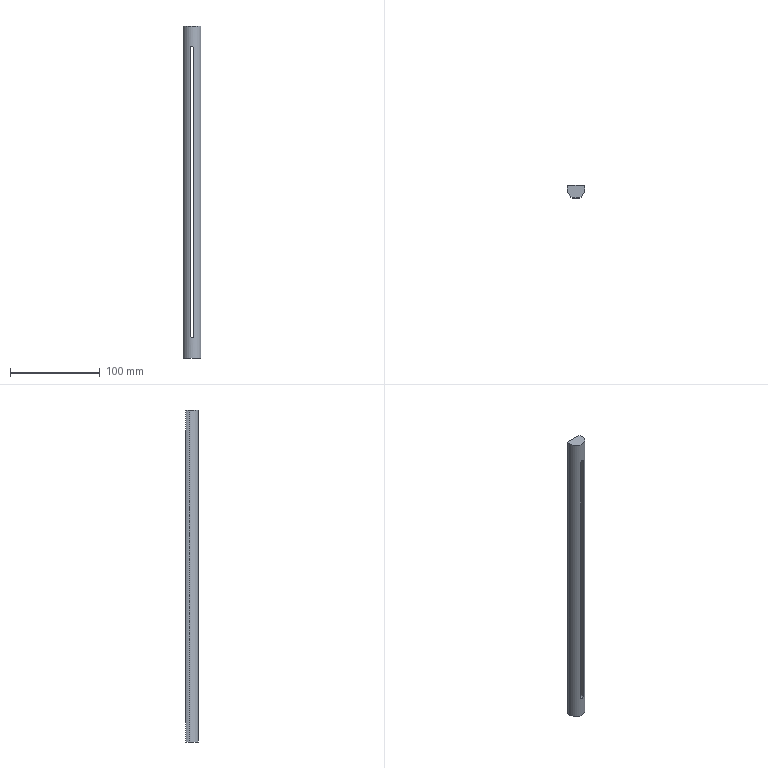Part | SolidWorks | features ICE 2, Extrusion 1 | 1 solid | 11 faces | box 20 x 14 x 370 mm | volume 68901 mm3 | cylinder 6 | plane 5 | commonest cylinder face diameters 4 x3 20 x3
STEP:
#1=CARTESIAN_POINT('',(0.,-10.,162.));
#2=VERTEX_POINT('',#1);
#3=CARTESIAN_POINT('',(2.,-9.798,160.));
#4=VERTEX_POINT('',#3);
#5=CARTESIAN_POINT('',(0.,-10.,162.));
#6=CARTESIAN_POINT('',(0.1307,-10.,162.));
#7=CARTESIAN_POINT('',(0.2635,-9.997,161.987));
#8=CARTESIAN_POINT('',(0.5201,-9.987,161.936));
#9=CARTESIAN_POINT('',(0.6448,-9.98,161.898));
#10=CARTESIAN_POINT('',(1.008,-9.952,161.747));
#11=CARTESIAN_POINT('',(1.228,-9.926,161.6));
#12=CARTESIAN_POINT('',(1.507,-9.886,161.322));
#13=CARTESIAN_POINT('',(1.589,-9.873,161.221));
#14=CARTESIAN_POINT('',(1.734,-9.849,161.005));
#15=CARTESIAN_POINT('',(1.797,-9.837,160.888));
#16=CARTESIAN_POINT('',(1.897,-9.819,160.646));
#17=CARTESIAN_POINT('',(1.935,-9.811,160.522));
#18=CARTESIAN_POINT('',(1.987,-9.801,160.265));
#19=CARTESIAN_POINT('',(2.,-9.798,160.132));
#20=CARTESIAN_POINT('',(2.,-9.798,160.));
#21=B_SPLINE_CURVE_WITH_KNOTS('',3,(#5,#6,#7,#8,#9,#10,#11,#12,#13,#14,#15,#16,#17,#18,#19,#20),.UNSPECIFIED.,.F.,.F.,(4,2,2,2,2,2,2,4),(0.003135,0.003527,0.003918,0.004701,0.005093,0.005484,0.005876,0.006267),.UNSPECIFIED.);
#22=EDGE_CURVE('',#2,#4,#21,.T.);
#23=ORIENTED_EDGE('',*,*,#22,.F.);
#24=CARTESIAN_POINT('',(0.,4.,162.));
#25=VERTEX_POINT('',#24);
#26=CARTESIAN_POINT('',(0.,-12.5,162.));
#27=DIRECTION('',(0.,1.,0.));
#28=VECTOR('',#27,1000.);
#29=LINE('',#26,#28);
#30=EDGE_CURVE('',#2,#25,#29,.T.);
#31=ORIENTED_EDGE('',*,*,#30,.T.);
#32=CARTESIAN_POINT('',(2.,4.,160.));
#33=VERTEX_POINT('',#32);
#34=CARTESIAN_POINT('',(0.,4.,160.));
#35=DIRECTION('',(0.,1.,0.));
#36=DIRECTION('',(0.,0.,-1.));
#37=AXIS2_PLACEMENT_3D('',#34,#35,#36);
#38=CIRCLE('',#37,2.);
#39=EDGE_CURVE('',#25,#33,#38,.T.);
#40=ORIENTED_EDGE('',*,*,#39,.T.);
#41=CARTESIAN_POINT('',(2.,-12.5,160.));
#42=DIRECTION('',(0.,1.,0.));
#43=VECTOR('',#42,1000.);
#44=LINE('',#41,#43);
#45=EDGE_CURVE('',#4,#33,#44,.T.);
#46=ORIENTED_EDGE('',*,*,#45,.F.);
#47=EDGE_LOOP('',(#23,#31,#40,#46));
#48=FACE_OUTER_BOUND('',#47,.T.);
#49=CARTESIAN_POINT('',(0.,-12.5,160.));
#50=DIRECTION('',(0.,1.,0.));
#51=DIRECTION('',(0.,0.,1.));
#52=AXIS2_PLACEMENT_3D('',#49,#50,#51);
#53=CYLINDRICAL_SURFACE('',#52,2.);
#54=ADVANCED_FACE('',(#48),#53,.F.);
#55=CARTESIAN_POINT('',(10.,0.,185.));
#56=VERTEX_POINT('',#55);
#57=CARTESIAN_POINT('',(9.165,4.,185.));
#58=VERTEX_POINT('',#57);
#59=CARTESIAN_POINT('',(0.,0.,185.));
#60=DIRECTION('',(0.,0.,1.));
#61=DIRECTION('',(1.,0.,0.));
#62=AXIS2_PLACEMENT_3D('',#59,#60,#61);
#63=CIRCLE('',#62,10.);
#64=EDGE_CURVE('',#56,#58,#63,.T.);
#65=ORIENTED_EDGE('',*,*,#64,.F.);
#66=CARTESIAN_POINT('',(10.,0.,-185.));
#67=VERTEX_POINT('',#66);
#68=CARTESIAN_POINT('',(10.,0.,185.));
#69=DIRECTION('',(0.,0.,-1.));
#70=VECTOR('',#69,1000.);
#71=LINE('',#68,#70);
#72=EDGE_CURVE('',#56,#67,#71,.T.);
#73=ORIENTED_EDGE('',*,*,#72,.T.);
#74=CARTESIAN_POINT('',(9.165,4.,-185.));
#75=VERTEX_POINT('',#74);
#76=CARTESIAN_POINT('',(0.,0.,-185.));
#77=DIRECTION('',(0.,0.,1.));
#78=DIRECTION('',(1.,0.,0.));
#79=AXIS2_PLACEMENT_3D('',#76,#77,#78);
#80=CIRCLE('',#79,10.);
#81=EDGE_CURVE('',#67,#75,#80,.T.);
#82=ORIENTED_EDGE('',*,*,#81,.T.);
#83=CARTESIAN_POINT('',(9.165,4.,185.));
#84=DIRECTION('',(0.,0.,1.));
#85=VECTOR('',#84,1000.);
#86=LINE('',#83,#85);
#87=EDGE_CURVE('',#75,#58,#86,.T.);
#88=ORIENTED_EDGE('',*,*,#87,.T.);
#89=EDGE_LOOP('',(#65,#73,#82,#88));
#90=FACE_OUTER_BOUND('',#89,.T.);
#91=CARTESIAN_POINT('',(0.,0.,185.));
#92=DIRECTION('',(0.,0.,-1.));
#93=DIRECTION('',(-1.,0.,0.));
#94=AXIS2_PLACEMENT_3D('',#91,#92,#93);
#95=CYLINDRICAL_SURFACE('',#94,10.);
#96=ADVANCED_FACE('',(#90),#95,.T.);
#97=ORIENTED_EDGE('',*,*,#72,.F.);
#98=CARTESIAN_POINT('',(-10.,0.,185.));
#99=VERTEX_POINT('',#98);
#100=CARTESIAN_POINT('',(0.,0.,185.));
#101=DIRECTION('',(0.,0.,1.));
#102=DIRECTION('',(1.,0.,0.));
#103=AXIS2_PLACEMENT_3D('',#100,#101,#102);
#104=CIRCLE('',#103,10.);
#105=EDGE_CURVE('',#99,#56,#104,.T.);
#106=ORIENTED_EDGE('',*,*,#105,.F.);
#107=CARTESIAN_POINT('',(-10.,0.,-185.));
#108=VERTEX_POINT('',#107);
#109=CARTESIAN_POINT('',(-10.,0.,185.));
#110=DIRECTION('',(0.,0.,-1.));
#111=VECTOR('',#110,1000.);
#112=LINE('',#109,#111);
#113=EDGE_CURVE('',#99,#108,#112,.T.);
#114=ORIENTED_EDGE('',*,*,#113,.T.);
#115=CARTESIAN_POINT('',(0.,0.,-185.));
#116=DIRECTION('',(0.,0.,1.));
#117=DIRECTION('',(1.,0.,0.));
#118=AXIS2_PLACEMENT_3D('',#115,#116,#117);
#119=CIRCLE('',#118,10.);
#120=EDGE_CURVE('',#108,#67,#119,.T.);
#121=ORIENTED_EDGE('',*,*,#120,.T.);
#122=EDGE_LOOP('',(#97,#106,#114,#121));
#123=FACE_OUTER_BOUND('',#122,.T.);
#124=CARTESIAN_POINT('',(-2.,-9.798,-160.));
#125=VERTEX_POINT('',#124);
#126=CARTESIAN_POINT('',(-2.,-9.798,160.));
#127=VERTEX_POINT('',#126);
#128=CARTESIAN_POINT('',(-2.,-9.798,185.));
#129=DIRECTION('',(0.,0.,1.));
#130=VECTOR('',#129,1000.);
#131=LINE('',#128,#130);
#132=EDGE_CURVE('',#125,#127,#131,.T.);
#133=ORIENTED_EDGE('',*,*,#132,.T.);
#134=CARTESIAN_POINT('',(-2.,-9.798,160.));
#135=CARTESIAN_POINT('',(-2.,-9.798,160.133));
#136=CARTESIAN_POINT('',(-1.987,-9.801,160.263));
#137=CARTESIAN_POINT('',(-1.936,-9.811,160.519));
#138=CARTESIAN_POINT('',(-1.897,-9.819,160.646));
#139=CARTESIAN_POINT('',(-1.797,-9.837,160.888));
#140=CARTESIAN_POINT('',(-1.735,-9.849,161.003));
#141=CARTESIAN_POINT('',(-1.59,-9.873,161.22));
#142=CARTESIAN_POINT('',(-1.506,-9.886,161.323));
#143=CARTESIAN_POINT('',(-1.23,-9.926,161.599));
#144=CARTESIAN_POINT('',(-1.007,-9.952,161.748));
#145=CARTESIAN_POINT('',(-0.5255,-9.989,161.947));
#146=CARTESIAN_POINT('',(-0.2617,-10.,162.));
#147=CARTESIAN_POINT('',(0.,-10.,162.));
#148=B_SPLINE_CURVE_WITH_KNOTS('',3,(#134,#135,#136,#137,#138,#139,#140,#141,#142,#143,#144,#145,#146,#147),.UNSPECIFIED.,.F.,.F.,(4,2,2,2,2,2,4),(0.,0.0003919,0.0007838,0.001176,0.001568,0.002351,0.003135),.UNSPECIFIED.);
#149=EDGE_CURVE('',#127,#2,#148,.T.);
#150=ORIENTED_EDGE('',*,*,#149,.T.);
#151=ORIENTED_EDGE('',*,*,#22,.T.);
#152=CARTESIAN_POINT('',(2.,-9.798,-160.));
#153=VERTEX_POINT('',#152);
#154=CARTESIAN_POINT('',(2.,-9.798,185.));
#155=DIRECTION('',(0.,0.,-1.));
#156=VECTOR('',#155,1000.);
#157=LINE('',#154,#156);
#158=EDGE_CURVE('',#4,#153,#157,.T.);
#159=ORIENTED_EDGE('',*,*,#158,.T.);
#160=CARTESIAN_POINT('',(2.,-9.798,-160.));
#161=CARTESIAN_POINT('',(2.,-9.798,-160.132));
#162=CARTESIAN_POINT('',(1.987,-9.801,-160.263));
#163=CARTESIAN_POINT('',(1.936,-9.811,-160.519));
#164=CARTESIAN_POINT('',(1.897,-9.818,-160.646));
#165=CARTESIAN_POINT('',(1.797,-9.837,-160.888));
#166=CARTESIAN_POINT('',(1.735,-9.849,-161.003));
#167=CARTESIAN_POINT('',(1.59,-9.873,-161.22));
#168=CARTESIAN_POINT('',(1.506,-9.886,-161.322));
#169=CARTESIAN_POINT('',(1.23,-9.926,-161.598));
#170=CARTESIAN_POINT('',(1.008,-9.952,-161.747));
#171=CARTESIAN_POINT('',(0.5268,-9.989,-161.947));
#172=CARTESIAN_POINT('',(0.2632,-10.,-162.));
#173=CARTESIAN_POINT('',(-0.1292,-10.,-162.));
#174=CARTESIAN_POINT('',(-0.262,-9.997,-161.987));
#175=CARTESIAN_POINT('',(-0.5188,-9.987,-161.936));
#176=CARTESIAN_POINT('',(-0.6436,-9.98,-161.898));
#177=CARTESIAN_POINT('',(-1.007,-9.952,-161.748));
#178=CARTESIAN_POINT('',(-1.228,-9.926,-161.601));
#179=CARTESIAN_POINT('',(-1.506,-9.886,-161.322));
#180=CARTESIAN_POINT('',(-1.589,-9.873,-161.221));
#181=CARTESIAN_POINT('',(-1.734,-9.849,-161.005));
#182=CARTESIAN_POINT('',(-1.797,-9.837,-160.888));
#183=CARTESIAN_POINT('',(-1.897,-9.819,-160.647));
#184=CARTESIAN_POINT('',(-1.935,-9.811,-160.522));
#185=CARTESIAN_POINT('',(-1.987,-9.801,-160.265));
#186=CARTESIAN_POINT('',(-2.,-9.798,-160.132));
#187=CARTESIAN_POINT('',(-2.,-9.798,-160.));
#188=B_SPLINE_CURVE_WITH_KNOTS('',3,(#160,#161,#162,#163,#164,#165,#166,#167,#168,#169,#170,#171,#172,#173,#174,#175,#176,#177,#178,#179,#180,#181,#182,#183,#184,#185,#186,#187),.UNSPECIFIED.,.F.,.F.,(4,2,2,2,2,2,2,2,2,2,2,2,2,4),(0.,0.0003917,0.0007834,0.001175,0.001567,0.00235,0.003134,0.003525,0.003917,0.0047,0.005092,0.005484,0.005875,0.006267),.UNSPECIFIED.);
#189=EDGE_CURVE('',#153,#125,#188,.T.);
#190=ORIENTED_EDGE('',*,*,#189,.T.);
#191=EDGE_LOOP('',(#133,#150,#151,#159,#190));
#192=FACE_BOUND('',#191,.T.);
#193=CARTESIAN_POINT('',(0.,0.,185.));
#194=DIRECTION('',(0.,0.,-1.));
#195=DIRECTION('',(-1.,0.,0.));
#196=AXIS2_PLACEMENT_3D('',#193,#194,#195);
#197=CYLINDRICAL_SURFACE('',#196,10.);
#198=ADVANCED_FACE('',(#123,#192),#197,.T.);
#199=ORIENTED_EDGE('',*,*,#113,.F.);
#200=CARTESIAN_POINT('',(-9.165,4.,185.));
#201=VERTEX_POINT('',#200);
#202=CARTESIAN_POINT('',(0.,0.,185.));
#203=DIRECTION('',(0.,0.,1.));
#204=DIRECTION('',(1.,0.,0.));
#205=AXIS2_PLACEMENT_3D('',#202,#203,#204);
#206=CIRCLE('',#205,10.);
#207=EDGE_CURVE('',#201,#99,#206,.T.);
#208=ORIENTED_EDGE('',*,*,#207,.F.);
#209=CARTESIAN_POINT('',(-9.165,4.,-185.));
#210=VERTEX_POINT('',#209);
#211=CARTESIAN_POINT('',(-9.165,4.,185.));
#212=DIRECTION('',(0.,0.,-1.));
#213=VECTOR('',#212,1000.);
#214=LINE('',#211,#213);
#215=EDGE_CURVE('',#201,#210,#214,.T.);
#216=ORIENTED_EDGE('',*,*,#215,.T.);
#217=CARTESIAN_POINT('',(0.,0.,-185.));
#218=DIRECTION('',(0.,0.,1.));
#219=DIRECTION('',(1.,0.,0.));
#220=AXIS2_PLACEMENT_3D('',#217,#218,#219);
#221=CIRCLE('',#220,10.);
#222=EDGE_CURVE('',#210,#108,#221,.T.);
#223=ORIENTED_EDGE('',*,*,#222,.T.);
#224=EDGE_LOOP('',(#199,#208,#216,#223));
#225=FACE_OUTER_BOUND('',#224,.T.);
#226=CARTESIAN_POINT('',(0.,0.,185.));
#227=DIRECTION('',(0.,0.,-1.));
#228=DIRECTION('',(-1.,0.,0.));
#229=AXIS2_PLACEMENT_3D('',#226,#227,#228);
#230=CYLINDRICAL_SURFACE('',#229,10.);
#231=ADVANCED_FACE('',(#225),#230,.T.);
#232=CARTESIAN_POINT('',(-10.,4.,185.));
#233=DIRECTION('',(1.,0.,0.));
#234=VECTOR('',#233,1000.);
#235=LINE('',#232,#234);
#236=EDGE_CURVE('',#201,#58,#235,.T.);
#237=ORIENTED_EDGE('',*,*,#236,.F.);
#238=ORIENTED_EDGE('',*,*,#207,.T.);
#239=ORIENTED_EDGE('',*,*,#105,.T.);
#240=ORIENTED_EDGE('',*,*,#64,.T.);
#241=EDGE_LOOP('',(#237,#238,#239,#240));
#242=FACE_OUTER_BOUND('',#241,.T.);
#243=CARTESIAN_POINT('',(0.,0.,185.));
#244=DIRECTION('',(0.,0.,1.));
#245=DIRECTION('',(1.,0.,0.));
#246=AXIS2_PLACEMENT_3D('',#243,#244,#245);
#247=PLANE('',#246);
#248=ADVANCED_FACE('',(#242),#247,.T.);
#249=ORIENTED_EDGE('',*,*,#222,.F.);
#250=CARTESIAN_POINT('',(-10.,4.,-185.));
#251=DIRECTION('',(1.,0.,0.));
#252=VECTOR('',#251,1000.);
#253=LINE('',#250,#252);
#254=EDGE_CURVE('',#210,#75,#253,.T.);
#255=ORIENTED_EDGE('',*,*,#254,.T.);
#256=ORIENTED_EDGE('',*,*,#81,.F.);
#257=ORIENTED_EDGE('',*,*,#120,.F.);
#258=EDGE_LOOP('',(#249,#255,#256,#257));
#259=FACE_OUTER_BOUND('',#258,.T.);
#260=CARTESIAN_POINT('',(0.,0.,-185.));
#261=DIRECTION('',(0.,0.,1.));
#262=DIRECTION('',(1.,0.,0.));
#263=AXIS2_PLACEMENT_3D('',#260,#261,#262);
#264=PLANE('',#263);
#265=ADVANCED_FACE('',(#259),#264,.F.);
#266=ORIENTED_EDGE('',*,*,#30,.F.);
#267=ORIENTED_EDGE('',*,*,#149,.F.);
#268=CARTESIAN_POINT('',(-2.,4.,160.));
#269=VERTEX_POINT('',#268);
#270=CARTESIAN_POINT('',(-2.,-12.5,160.));
#271=DIRECTION('',(0.,1.,0.));
#272=VECTOR('',#271,1000.);
#273=LINE('',#270,#272);
#274=EDGE_CURVE('',#127,#269,#273,.T.);
#275=ORIENTED_EDGE('',*,*,#274,.T.);
#276=CARTESIAN_POINT('',(0.,4.,160.));
#277=DIRECTION('',(0.,1.,0.));
#278=DIRECTION('',(0.,0.,-1.));
#279=AXIS2_PLACEMENT_3D('',#276,#277,#278);
#280=CIRCLE('',#279,2.);
#281=EDGE_CURVE('',#269,#25,#280,.T.);
#282=ORIENTED_EDGE('',*,*,#281,.T.);
#283=EDGE_LOOP('',(#266,#267,#275,#282));
#284=FACE_OUTER_BOUND('',#283,.T.);
#285=CARTESIAN_POINT('',(0.,-12.5,160.));
#286=DIRECTION('',(0.,1.,0.));
#287=DIRECTION('',(0.,0.,1.));
#288=AXIS2_PLACEMENT_3D('',#285,#286,#287);
#289=CYLINDRICAL_SURFACE('',#288,2.);
#290=ADVANCED_FACE('',(#284),#289,.F.);
#291=CARTESIAN_POINT('',(-2.,4.,-160.));
#292=VERTEX_POINT('',#291);
#293=CARTESIAN_POINT('',(-2.,-12.5,-160.));
#294=DIRECTION('',(0.,1.,0.));
#295=VECTOR('',#294,1000.);
#296=LINE('',#293,#295);
#297=EDGE_CURVE('',#125,#292,#296,.T.);
#298=ORIENTED_EDGE('',*,*,#297,.T.);
#299=CARTESIAN_POINT('',(-2.,4.,160.));
#300=DIRECTION('',(0.,0.,1.));
#301=VECTOR('',#300,1000.);
#302=LINE('',#299,#301);
#303=EDGE_CURVE('',#292,#269,#302,.T.);
#304=ORIENTED_EDGE('',*,*,#303,.T.);
#305=ORIENTED_EDGE('',*,*,#274,.F.);
#306=ORIENTED_EDGE('',*,*,#132,.F.);
#307=EDGE_LOOP('',(#298,#304,#305,#306));
#308=FACE_OUTER_BOUND('',#307,.T.);
#309=CARTESIAN_POINT('',(-2.,-12.5,160.));
#310=DIRECTION('',(-1.,0.,0.));
#311=DIRECTION('',(0.,0.,1.));
#312=AXIS2_PLACEMENT_3D('',#309,#310,#311);
#313=PLANE('',#312);
#314=ADVANCED_FACE('',(#308),#313,.F.);
#315=CARTESIAN_POINT('',(2.,4.,-160.));
#316=VERTEX_POINT('',#315);
#317=CARTESIAN_POINT('',(2.,-12.5,-160.));
#318=DIRECTION('',(0.,1.,0.));
#319=VECTOR('',#318,1000.);
#320=LINE('',#317,#319);
#321=EDGE_CURVE('',#153,#316,#320,.T.);
#322=ORIENTED_EDGE('',*,*,#321,.T.);
#323=CARTESIAN_POINT('',(0.,4.,-160.));
#324=DIRECTION('',(0.,1.,0.));
#325=DIRECTION('',(0.,0.,-1.));
#326=AXIS2_PLACEMENT_3D('',#323,#324,#325);
#327=CIRCLE('',#326,2.);
#328=EDGE_CURVE('',#316,#292,#327,.T.);
#329=ORIENTED_EDGE('',*,*,#328,.T.);
#330=ORIENTED_EDGE('',*,*,#297,.F.);
#331=ORIENTED_EDGE('',*,*,#189,.F.);
#332=EDGE_LOOP('',(#322,#329,#330,#331));
#333=FACE_OUTER_BOUND('',#332,.T.);
#334=CARTESIAN_POINT('',(0.,-12.5,-160.));
#335=DIRECTION('',(0.,1.,0.));
#336=DIRECTION('',(0.,0.,1.));
#337=AXIS2_PLACEMENT_3D('',#334,#335,#336);
#338=CYLINDRICAL_SURFACE('',#337,2.);
#339=ADVANCED_FACE('',(#333),#338,.F.);
#340=ORIENTED_EDGE('',*,*,#45,.T.);
#341=CARTESIAN_POINT('',(2.,4.,160.));
#342=DIRECTION('',(0.,0.,-1.));
#343=VECTOR('',#342,1000.);
#344=LINE('',#341,#343);
#345=EDGE_CURVE('',#33,#316,#344,.T.);
#346=ORIENTED_EDGE('',*,*,#345,.T.);
#347=ORIENTED_EDGE('',*,*,#321,.F.);
#348=ORIENTED_EDGE('',*,*,#158,.F.);
#349=EDGE_LOOP('',(#340,#346,#347,#348));
#350=FACE_OUTER_BOUND('',#349,.T.);
#351=CARTESIAN_POINT('',(2.,-12.5,160.));
#352=DIRECTION('',(1.,0.,0.));
#353=DIRECTION('',(0.,0.,-1.));
#354=AXIS2_PLACEMENT_3D('',#351,#352,#353);
#355=PLANE('',#354);
#356=ADVANCED_FACE('',(#350),#355,.F.);
#357=ORIENTED_EDGE('',*,*,#303,.F.);
#358=ORIENTED_EDGE('',*,*,#328,.F.);
#359=ORIENTED_EDGE('',*,*,#345,.F.);
#360=ORIENTED_EDGE('',*,*,#39,.F.);
#361=ORIENTED_EDGE('',*,*,#281,.F.);
#362=EDGE_LOOP('',(#357,#358,#359,#360,#361));
#363=FACE_BOUND('',#362,.T.);
#364=ORIENTED_EDGE('',*,*,#236,.T.);
#365=ORIENTED_EDGE('',*,*,#87,.F.);
#366=ORIENTED_EDGE('',*,*,#254,.F.);
#367=ORIENTED_EDGE('',*,*,#215,.F.);
#368=EDGE_LOOP('',(#364,#365,#366,#367));
#369=FACE_OUTER_BOUND('',#368,.T.);
#370=CARTESIAN_POINT('',(-10.,4.,185.));
#371=DIRECTION('',(0.,-1.,0.));
#372=DIRECTION('',(0.,0.,-1.));
#373=AXIS2_PLACEMENT_3D('',#370,#371,#372);
#374=PLANE('',#373);
#375=ADVANCED_FACE('',(#363,#369),#374,.F.);
#376=CLOSED_SHELL('',(#54,#96,#198,#231,#248,#265,#290,#314,#339,#356,#375));
#377=MANIFOLD_SOLID_BREP('',#376);
#378=CARTESIAN_POINT('',(0.,0.,0.));
#379=DIRECTION('',(0.,0.,1.));
#380=DIRECTION('',(1.,0.,0.));
#381=AXIS2_PLACEMENT_3D('',#378,#379,#380);
#382=(LENGTH_UNIT()NAMED_UNIT(*)SI_UNIT(.MILLI.,.METRE.));
#383=UNCERTAINTY_MEASURE_WITH_UNIT(LENGTH_MEASURE(0.00001),#382,'','');
#384=(NAMED_UNIT(*)PLANE_ANGLE_UNIT()SI_UNIT($,.RADIAN.));
#385=(NAMED_UNIT(*)SI_UNIT($,.STERADIAN.)SOLID_ANGLE_UNIT());
#386=(GEOMETRIC_REPRESENTATION_CONTEXT(3)GLOBAL_UNCERTAINTY_ASSIGNED_CONTEXT((#383))GLOBAL_UNIT_ASSIGNED_CONTEXT((#382,#384,#385))REPRESENTATION_CONTEXT('',''));
#387=ADVANCED_BREP_SHAPE_REPRESENTATION('',(#377,#381),#386);